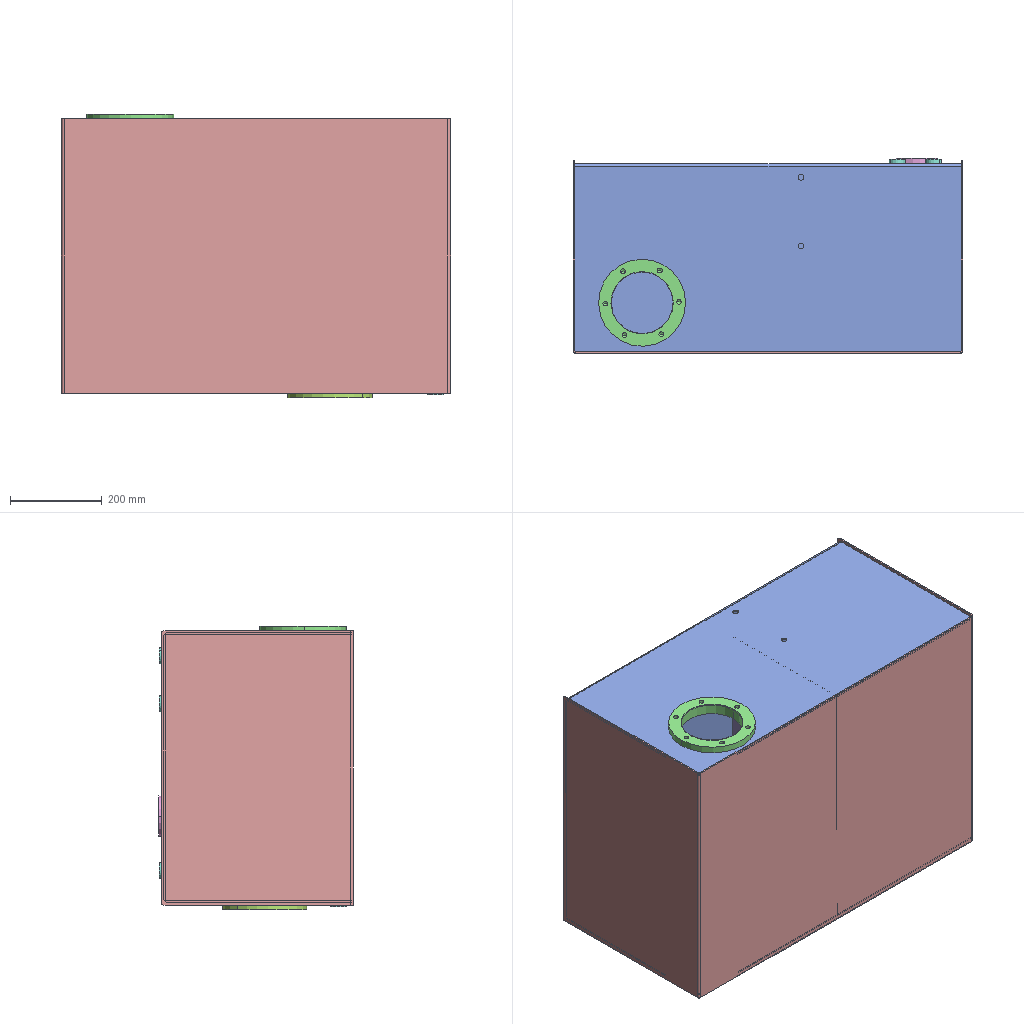Assembly | SolidWorks | 9 different items | 19 placed | box 850 x 426 x 620 mm
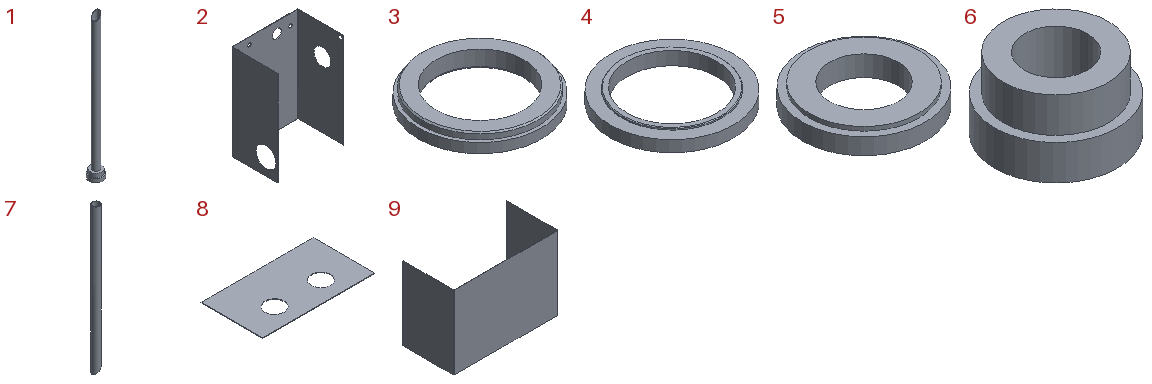Parts list (item | name | quantity | parent item | size | volume | features):
1 | (subassembly) | x4 | - | 35 x 35 x 370 mm | 29813 mm3 | features CompositeCurve 2
2 | - | x1 | - | 588 x 411 x 844 mm | 3388584 mm3 | features ICE 4, FlatPattern 1, SMBaseFlange 1, SheetMetal 1
3 | - | x1 | - | 190 x 190 x 25 mm | 309604 mm3 | features Chamfer 2, 3DProfileFeature 1, Extrusion 1, HoleWzd 1, ICE 1
4 | - | x1 | - | 185 x 185 x 20 mm | 216002 mm3 | features Fillet 2, ICE 2, 3DProfileFeature 1, Chamfer 1, Extrusion 1, HoleWzd 1
5 | - | x1 | - | 90 x 90 x 15 mm | 61433 mm3 | features 3DProfileFeature 1, Extrusion 1, HoleWzd 1, ICE 1
6 | - | x5 | in 1 | 35 x 35 x 20 mm | 11600 mm3 | features ICE 2, Extrusion 1
7 | - | x4 | in 1 | 18 x 18 x 350 mm | 18212 mm3 | features Extrusion 1, ICE 1
8 | - | x1 | - | 582 x 320 x 3 mm | 511596 mm3 | features FlatPattern 1, SMBaseFlange 1, SheetMetal 1
9 | - | x1 | - | 850 x 420 x 600 mm | 3024154 mm3 | features FlatPattern 1, ICE 1, SMBaseFlange 1, SheetMetal 1
Mates (type | each side: item.copy, entity, surface, feature):
In the top assembly
Coincident | 9.1 face plane Base-Flange1 | 2.1 face plane Base-Flange1 | 2 times
DistanceDim | 2.1 face plane Base-Flange1 | 9.1 face plane Base-Flange1
Concentric | 2.1 edge | 4.1 edge
Coincident | 2.1 face plane Base-Flange1 | 4.1 face plane Boss-Extrude1
Concentric | 2.1 edge | 5.1 edge
Coincident | 2.1 face plane Base-Flange1 | 5.1 face plane Boss-Extrude1
Concentric | 2.1 edge | 6.1 edge
Coincident | 2.1 face plane Base-Flange1 | 6.1 face plane Boss-Extrude1
Concentric | 2.1 edge | 6.2 edge
Coincident | 2.1 face plane Base-Flange1 | 6.2 face plane Boss-Extrude1
Concentric | 2.1 edge | 6.3 edge
Coincident | 2.1 face plane Base-Flange1 | 6.3 face plane Boss-Extrude1
Concentric | 2.1 edge | 6.4 edge
Coincident | 2.1 face plane Base-Flange1 | 6.4 face plane Boss-Extrude1
Concentric | 2.1 edge | 6.5 edge
Coincident | 2.1 face plane Base-Flange1 | 6.5 face plane Boss-Extrude1
Concentric | 2.1 edge | 3.1 edge
Coincident | 2.1 face plane Base-Flange1 | 3.1 face plane Boss-Extrude1
Coincident | 9.1 face plane Base-Flange1 | 8.1 face plane Base-Flange1
DistanceDim | 8.1 face plane Base-Flange1 | 9.1 face plane Base-Flange1
Coincident | 2.1 face plane Base-Flange1 | 8.1 face plane Base-Flange1
In subassembly 1
Concentric | 7.1 edge | 6.1 edge
DistanceDim | 7.1 face plane Boss-Extrude1 | 6.1 face plane Boss-Extrude1